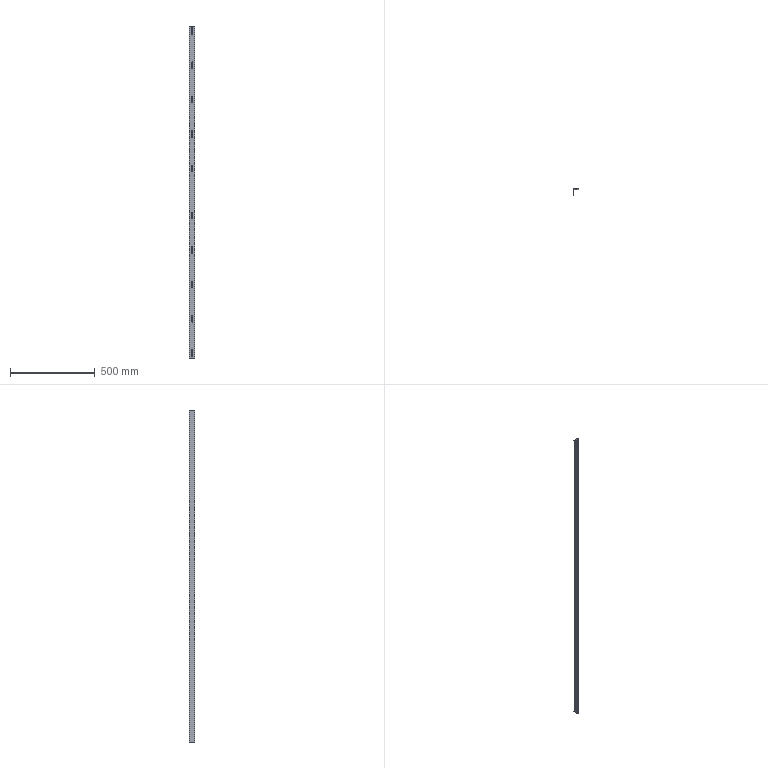Part | 1 solid | 64 faces | box 35 x 35 x 1956 mm | volume 194421 mm3 | cylinder 32 | plane 32 | commonest cylinder face diameters 8 x30 2 x1 5 x1